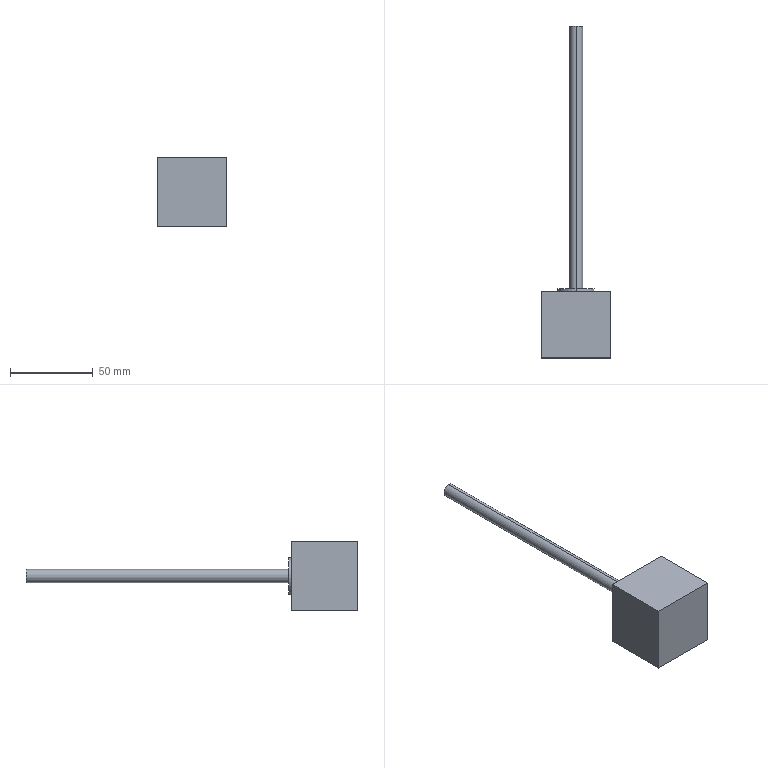Part | SolidWorks | features ICE 3, Extrusion 1, HoleWzd 1 | 1 solid | 28 faces | box 42 x 201 x 42 mm | volume 79160 mm3 | cylinder 12 | cone 8 | plane 8 | commonest cylinder face diameters 2.5 x8 8 x2 22 x2
STEP:
#1=CARTESIAN_POINT('',(-15.5,32.5,-16.75));
#2=VERTEX_POINT('',#1);
#3=CARTESIAN_POINT('',(-15.5,32.5,-14.25));
#4=VERTEX_POINT('',#3);
#5=CARTESIAN_POINT('',(-15.5,32.5,-15.5));
#6=DIRECTION('',(0.,1.,0.));
#7=DIRECTION('',(0.,0.,1.));
#8=AXIS2_PLACEMENT_3D('',#5,#6,#7);
#9=CIRCLE('',#8,1.25);
#10=EDGE_CURVE('',#2,#4,#9,.T.);
#11=ORIENTED_EDGE('',*,*,#10,.F.);
#12=CARTESIAN_POINT('',(-15.5,40.,-16.75));
#13=VERTEX_POINT('',#12);
#14=CARTESIAN_POINT('',(-15.5,40.,-16.75));
#15=DIRECTION('',(0.,1.,0.));
#16=VECTOR('',#15,1000.);
#17=LINE('',#14,#16);
#18=EDGE_CURVE('',#2,#13,#17,.T.);
#19=ORIENTED_EDGE('',*,*,#18,.T.);
#20=CARTESIAN_POINT('',(-15.5,40.,-14.25));
#21=VERTEX_POINT('',#20);
#22=CARTESIAN_POINT('',(-15.5,40.,-15.5));
#23=DIRECTION('',(0.,1.,0.));
#24=DIRECTION('',(0.,0.,1.));
#25=AXIS2_PLACEMENT_3D('',#22,#23,#24);
#26=CIRCLE('',#25,1.25);
#27=EDGE_CURVE('',#13,#21,#26,.T.);
#28=ORIENTED_EDGE('',*,*,#27,.T.);
#29=CARTESIAN_POINT('',(-15.5,40.,-14.25));
#30=DIRECTION('',(0.,1.,0.));
#31=VECTOR('',#30,1000.);
#32=LINE('',#29,#31);
#33=EDGE_CURVE('',#4,#21,#32,.T.);
#34=ORIENTED_EDGE('',*,*,#33,.F.);
#35=EDGE_LOOP('',(#11,#19,#28,#34));
#36=FACE_OUTER_BOUND('',#35,.T.);
#37=CARTESIAN_POINT('',(-15.5,40.,-15.5));
#38=DIRECTION('',(0.,1.,0.));
#39=DIRECTION('',(0.,0.,1.));
#40=AXIS2_PLACEMENT_3D('',#37,#38,#39);
#41=CYLINDRICAL_SURFACE('',#40,1.25);
#42=ADVANCED_FACE('',(#36),#41,.F.);
#43=CARTESIAN_POINT('',(-15.5,31.749,-15.5));
#44=VERTEX_POINT('',#43);
#45=CARTESIAN_POINT('',(-15.5,32.5,-14.25));
#46=DIRECTION('',(0.,0.515,0.8572));
#47=VECTOR('',#46,1000.);
#48=LINE('',#45,#47);
#49=EDGE_CURVE('',#44,#4,#48,.T.);
#50=ORIENTED_EDGE('',*,*,#49,.F.);
#51=CARTESIAN_POINT('',(-15.5,32.5,-16.75));
#52=DIRECTION('',(0.,0.515,-0.8572));
#53=VECTOR('',#52,1000.);
#54=LINE('',#51,#53);
#55=EDGE_CURVE('',#44,#2,#54,.T.);
#56=ORIENTED_EDGE('',*,*,#55,.T.);
#57=ORIENTED_EDGE('',*,*,#10,.T.);
#58=EDGE_LOOP('',(#50,#56,#57));
#59=FACE_OUTER_BOUND('',#58,.T.);
#60=CARTESIAN_POINT('',(-15.5,32.5,-15.5));
#61=DIRECTION('',(0.,1.,0.));
#62=DIRECTION('',(0.,0.,1.));
#63=AXIS2_PLACEMENT_3D('',#60,#61,#62);
#64=CONICAL_SURFACE('',#63,1.25,1.03);
#65=ADVANCED_FACE('',(#59),#64,.F.);
#66=CARTESIAN_POINT('',(15.5,32.5,14.25));
#67=VERTEX_POINT('',#66);
#68=CARTESIAN_POINT('',(15.5,32.5,16.75));
#69=VERTEX_POINT('',#68);
#70=CARTESIAN_POINT('',(15.5,32.5,15.5));
#71=DIRECTION('',(0.,1.,0.));
#72=DIRECTION('',(0.,0.,1.));
#73=AXIS2_PLACEMENT_3D('',#70,#71,#72);
#74=CIRCLE('',#73,1.25);
#75=EDGE_CURVE('',#67,#69,#74,.T.);
#76=ORIENTED_EDGE('',*,*,#75,.F.);
#77=CARTESIAN_POINT('',(15.5,40.,14.25));
#78=VERTEX_POINT('',#77);
#79=CARTESIAN_POINT('',(15.5,40.,14.25));
#80=DIRECTION('',(0.,1.,0.));
#81=VECTOR('',#80,1000.);
#82=LINE('',#79,#81);
#83=EDGE_CURVE('',#67,#78,#82,.T.);
#84=ORIENTED_EDGE('',*,*,#83,.T.);
#85=CARTESIAN_POINT('',(15.5,40.,16.75));
#86=VERTEX_POINT('',#85);
#87=CARTESIAN_POINT('',(15.5,40.,15.5));
#88=DIRECTION('',(0.,1.,0.));
#89=DIRECTION('',(0.,0.,1.));
#90=AXIS2_PLACEMENT_3D('',#87,#88,#89);
#91=CIRCLE('',#90,1.25);
#92=EDGE_CURVE('',#78,#86,#91,.T.);
#93=ORIENTED_EDGE('',*,*,#92,.T.);
#94=CARTESIAN_POINT('',(15.5,40.,16.75));
#95=DIRECTION('',(0.,1.,0.));
#96=VECTOR('',#95,1000.);
#97=LINE('',#94,#96);
#98=EDGE_CURVE('',#69,#86,#97,.T.);
#99=ORIENTED_EDGE('',*,*,#98,.F.);
#100=EDGE_LOOP('',(#76,#84,#93,#99));
#101=FACE_OUTER_BOUND('',#100,.T.);
#102=CARTESIAN_POINT('',(15.5,40.,15.5));
#103=DIRECTION('',(0.,1.,0.));
#104=DIRECTION('',(0.,0.,1.));
#105=AXIS2_PLACEMENT_3D('',#102,#103,#104);
#106=CYLINDRICAL_SURFACE('',#105,1.25);
#107=ADVANCED_FACE('',(#101),#106,.F.);
#108=CARTESIAN_POINT('',(15.5,31.749,15.5));
#109=VERTEX_POINT('',#108);
#110=CARTESIAN_POINT('',(15.5,32.5,16.75));
#111=DIRECTION('',(0.,0.515,0.8572));
#112=VECTOR('',#111,1000.);
#113=LINE('',#110,#112);
#114=EDGE_CURVE('',#109,#69,#113,.T.);
#115=ORIENTED_EDGE('',*,*,#114,.F.);
#116=CARTESIAN_POINT('',(15.5,32.5,14.25));
#117=DIRECTION('',(0.,0.515,-0.8572));
#118=VECTOR('',#117,1000.);
#119=LINE('',#116,#118);
#120=EDGE_CURVE('',#109,#67,#119,.T.);
#121=ORIENTED_EDGE('',*,*,#120,.T.);
#122=ORIENTED_EDGE('',*,*,#75,.T.);
#123=EDGE_LOOP('',(#115,#121,#122));
#124=FACE_OUTER_BOUND('',#123,.T.);
#125=CARTESIAN_POINT('',(15.5,32.5,15.5));
#126=DIRECTION('',(0.,1.,0.));
#127=DIRECTION('',(0.,0.,1.));
#128=AXIS2_PLACEMENT_3D('',#125,#126,#127);
#129=CONICAL_SURFACE('',#128,1.25,1.03);
#130=ADVANCED_FACE('',(#124),#129,.F.);
#131=CARTESIAN_POINT('',(-15.5,32.5,14.25));
#132=VERTEX_POINT('',#131);
#133=CARTESIAN_POINT('',(-15.5,32.5,16.75));
#134=VERTEX_POINT('',#133);
#135=CARTESIAN_POINT('',(-15.5,32.5,15.5));
#136=DIRECTION('',(0.,1.,0.));
#137=DIRECTION('',(0.,0.,1.));
#138=AXIS2_PLACEMENT_3D('',#135,#136,#137);
#139=CIRCLE('',#138,1.25);
#140=EDGE_CURVE('',#132,#134,#139,.T.);
#141=ORIENTED_EDGE('',*,*,#140,.F.);
#142=CARTESIAN_POINT('',(-15.5,40.,14.25));
#143=VERTEX_POINT('',#142);
#144=CARTESIAN_POINT('',(-15.5,40.,14.25));
#145=DIRECTION('',(0.,1.,0.));
#146=VECTOR('',#145,1000.);
#147=LINE('',#144,#146);
#148=EDGE_CURVE('',#132,#143,#147,.T.);
#149=ORIENTED_EDGE('',*,*,#148,.T.);
#150=CARTESIAN_POINT('',(-15.5,40.,16.75));
#151=VERTEX_POINT('',#150);
#152=CARTESIAN_POINT('',(-15.5,40.,15.5));
#153=DIRECTION('',(0.,1.,0.));
#154=DIRECTION('',(0.,0.,1.));
#155=AXIS2_PLACEMENT_3D('',#152,#153,#154);
#156=CIRCLE('',#155,1.25);
#157=EDGE_CURVE('',#143,#151,#156,.T.);
#158=ORIENTED_EDGE('',*,*,#157,.T.);
#159=CARTESIAN_POINT('',(-15.5,40.,16.75));
#160=DIRECTION('',(0.,1.,0.));
#161=VECTOR('',#160,1000.);
#162=LINE('',#159,#161);
#163=EDGE_CURVE('',#134,#151,#162,.T.);
#164=ORIENTED_EDGE('',*,*,#163,.F.);
#165=EDGE_LOOP('',(#141,#149,#158,#164));
#166=FACE_OUTER_BOUND('',#165,.T.);
#167=CARTESIAN_POINT('',(-15.5,40.,15.5));
#168=DIRECTION('',(0.,1.,0.));
#169=DIRECTION('',(0.,0.,1.));
#170=AXIS2_PLACEMENT_3D('',#167,#168,#169);
#171=CYLINDRICAL_SURFACE('',#170,1.25);
#172=ADVANCED_FACE('',(#166),#171,.F.);
#173=CARTESIAN_POINT('',(-15.5,31.749,15.5));
#174=VERTEX_POINT('',#173);
#175=CARTESIAN_POINT('',(-15.5,32.5,16.75));
#176=DIRECTION('',(0.,0.515,0.8572));
#177=VECTOR('',#176,1000.);
#178=LINE('',#175,#177);
#179=EDGE_CURVE('',#174,#134,#178,.T.);
#180=ORIENTED_EDGE('',*,*,#179,.F.);
#181=CARTESIAN_POINT('',(-15.5,32.5,14.25));
#182=DIRECTION('',(0.,0.515,-0.8572));
#183=VECTOR('',#182,1000.);
#184=LINE('',#181,#183);
#185=EDGE_CURVE('',#174,#132,#184,.T.);
#186=ORIENTED_EDGE('',*,*,#185,.T.);
#187=ORIENTED_EDGE('',*,*,#140,.T.);
#188=EDGE_LOOP('',(#180,#186,#187));
#189=FACE_OUTER_BOUND('',#188,.T.);
#190=CARTESIAN_POINT('',(-15.5,32.5,15.5));
#191=DIRECTION('',(0.,1.,0.));
#192=DIRECTION('',(0.,0.,1.));
#193=AXIS2_PLACEMENT_3D('',#190,#191,#192);
#194=CONICAL_SURFACE('',#193,1.25,1.03);
#195=ADVANCED_FACE('',(#189),#194,.F.);
#196=CARTESIAN_POINT('',(15.5,32.5,-16.75));
#197=VERTEX_POINT('',#196);
#198=CARTESIAN_POINT('',(15.5,32.5,-14.25));
#199=VERTEX_POINT('',#198);
#200=CARTESIAN_POINT('',(15.5,32.5,-15.5));
#201=DIRECTION('',(0.,1.,0.));
#202=DIRECTION('',(0.,0.,1.));
#203=AXIS2_PLACEMENT_3D('',#200,#201,#202);
#204=CIRCLE('',#203,1.25);
#205=EDGE_CURVE('',#197,#199,#204,.T.);
#206=ORIENTED_EDGE('',*,*,#205,.F.);
#207=CARTESIAN_POINT('',(15.5,40.,-16.75));
#208=VERTEX_POINT('',#207);
#209=CARTESIAN_POINT('',(15.5,40.,-16.75));
#210=DIRECTION('',(0.,1.,0.));
#211=VECTOR('',#210,1000.);
#212=LINE('',#209,#211);
#213=EDGE_CURVE('',#197,#208,#212,.T.);
#214=ORIENTED_EDGE('',*,*,#213,.T.);
#215=CARTESIAN_POINT('',(15.5,40.,-14.25));
#216=VERTEX_POINT('',#215);
#217=CARTESIAN_POINT('',(15.5,40.,-15.5));
#218=DIRECTION('',(0.,1.,0.));
#219=DIRECTION('',(0.,0.,1.));
#220=AXIS2_PLACEMENT_3D('',#217,#218,#219);
#221=CIRCLE('',#220,1.25);
#222=EDGE_CURVE('',#208,#216,#221,.T.);
#223=ORIENTED_EDGE('',*,*,#222,.T.);
#224=CARTESIAN_POINT('',(15.5,40.,-14.25));
#225=DIRECTION('',(0.,1.,0.));
#226=VECTOR('',#225,1000.);
#227=LINE('',#224,#226);
#228=EDGE_CURVE('',#199,#216,#227,.T.);
#229=ORIENTED_EDGE('',*,*,#228,.F.);
#230=EDGE_LOOP('',(#206,#214,#223,#229));
#231=FACE_OUTER_BOUND('',#230,.T.);
#232=CARTESIAN_POINT('',(15.5,40.,-15.5));
#233=DIRECTION('',(0.,1.,0.));
#234=DIRECTION('',(0.,0.,1.));
#235=AXIS2_PLACEMENT_3D('',#232,#233,#234);
#236=CYLINDRICAL_SURFACE('',#235,1.25);
#237=ADVANCED_FACE('',(#231),#236,.F.);
#238=CARTESIAN_POINT('',(15.5,31.749,-15.5));
#239=VERTEX_POINT('',#238);
#240=CARTESIAN_POINT('',(15.5,32.5,-14.25));
#241=DIRECTION('',(0.,0.515,0.8572));
#242=VECTOR('',#241,1000.);
#243=LINE('',#240,#242);
#244=EDGE_CURVE('',#239,#199,#243,.T.);
#245=ORIENTED_EDGE('',*,*,#244,.F.);
#246=CARTESIAN_POINT('',(15.5,32.5,-16.75));
#247=DIRECTION('',(0.,0.515,-0.8572));
#248=VECTOR('',#247,1000.);
#249=LINE('',#246,#248);
#250=EDGE_CURVE('',#239,#197,#249,.T.);
#251=ORIENTED_EDGE('',*,*,#250,.T.);
#252=ORIENTED_EDGE('',*,*,#205,.T.);
#253=EDGE_LOOP('',(#245,#251,#252));
#254=FACE_OUTER_BOUND('',#253,.T.);
#255=CARTESIAN_POINT('',(15.5,32.5,-15.5));
#256=DIRECTION('',(0.,1.,0.));
#257=DIRECTION('',(0.,0.,1.));
#258=AXIS2_PLACEMENT_3D('',#255,#256,#257);
#259=CONICAL_SURFACE('',#258,1.25,1.03);
#260=ADVANCED_FACE('',(#254),#259,.F.);
#261=CARTESIAN_POINT('',(0.,201.,4.));
#262=VERTEX_POINT('',#261);
#263=CARTESIAN_POINT('',(0.,201.,-4.));
#264=VERTEX_POINT('',#263);
#265=CARTESIAN_POINT('',(0.,201.,0.));
#266=DIRECTION('',(0.,1.,0.));
#267=DIRECTION('',(0.,0.,1.));
#268=AXIS2_PLACEMENT_3D('',#265,#266,#267);
#269=CIRCLE('',#268,4.);
#270=EDGE_CURVE('',#262,#264,#269,.T.);
#271=ORIENTED_EDGE('',*,*,#270,.F.);
#272=CARTESIAN_POINT('',(0.,42.,4.));
#273=VERTEX_POINT('',#272);
#274=CARTESIAN_POINT('',(0.,201.,4.));
#275=DIRECTION('',(0.,-1.,0.));
#276=VECTOR('',#275,1000.);
#277=LINE('',#274,#276);
#278=EDGE_CURVE('',#262,#273,#277,.T.);
#279=ORIENTED_EDGE('',*,*,#278,.T.);
#280=CARTESIAN_POINT('',(0.,42.,-4.));
#281=VERTEX_POINT('',#280);
#282=CARTESIAN_POINT('',(0.,42.,0.));
#283=DIRECTION('',(0.,1.,0.));
#284=DIRECTION('',(0.,0.,1.));
#285=AXIS2_PLACEMENT_3D('',#282,#283,#284);
#286=CIRCLE('',#285,4.);
#287=EDGE_CURVE('',#273,#281,#286,.T.);
#288=ORIENTED_EDGE('',*,*,#287,.T.);
#289=CARTESIAN_POINT('',(0.,201.,-4.));
#290=DIRECTION('',(0.,-1.,0.));
#291=VECTOR('',#290,1000.);
#292=LINE('',#289,#291);
#293=EDGE_CURVE('',#264,#281,#292,.T.);
#294=ORIENTED_EDGE('',*,*,#293,.F.);
#295=EDGE_LOOP('',(#271,#279,#288,#294));
#296=FACE_OUTER_BOUND('',#295,.T.);
#297=CARTESIAN_POINT('',(0.,201.,0.));
#298=DIRECTION('',(0.,-1.,0.));
#299=DIRECTION('',(0.,0.,-1.));
#300=AXIS2_PLACEMENT_3D('',#297,#298,#299);
#301=CYLINDRICAL_SURFACE('',#300,4.);
#302=ADVANCED_FACE('',(#296),#301,.T.);
#303=CARTESIAN_POINT('',(0.,42.,11.));
#304=VERTEX_POINT('',#303);
#305=CARTESIAN_POINT('',(0.,42.,-11.));
#306=VERTEX_POINT('',#305);
#307=CARTESIAN_POINT('',(0.,42.,0.));
#308=DIRECTION('',(0.,1.,0.));
#309=DIRECTION('',(0.,0.,1.));
#310=AXIS2_PLACEMENT_3D('',#307,#308,#309);
#311=CIRCLE('',#310,11.);
#312=EDGE_CURVE('',#304,#306,#311,.T.);
#313=ORIENTED_EDGE('',*,*,#312,.F.);
#314=CARTESIAN_POINT('',(0.,40.,11.));
#315=VERTEX_POINT('',#314);
#316=CARTESIAN_POINT('',(0.,42.,11.));
#317=DIRECTION('',(0.,-1.,0.));
#318=VECTOR('',#317,1000.);
#319=LINE('',#316,#318);
#320=EDGE_CURVE('',#304,#315,#319,.T.);
#321=ORIENTED_EDGE('',*,*,#320,.T.);
#322=CARTESIAN_POINT('',(0.,40.,-11.));
#323=VERTEX_POINT('',#322);
#324=CARTESIAN_POINT('',(0.,40.,0.));
#325=DIRECTION('',(0.,1.,0.));
#326=DIRECTION('',(0.,0.,1.));
#327=AXIS2_PLACEMENT_3D('',#324,#325,#326);
#328=CIRCLE('',#327,11.);
#329=EDGE_CURVE('',#315,#323,#328,.T.);
#330=ORIENTED_EDGE('',*,*,#329,.T.);
#331=CARTESIAN_POINT('',(0.,42.,-11.));
#332=DIRECTION('',(0.,-1.,0.));
#333=VECTOR('',#332,1000.);
#334=LINE('',#331,#333);
#335=EDGE_CURVE('',#306,#323,#334,.T.);
#336=ORIENTED_EDGE('',*,*,#335,.F.);
#337=EDGE_LOOP('',(#313,#321,#330,#336));
#338=FACE_OUTER_BOUND('',#337,.T.);
#339=CARTESIAN_POINT('',(0.,42.,0.));
#340=DIRECTION('',(0.,-1.,0.));
#341=DIRECTION('',(0.,0.,-1.));
#342=AXIS2_PLACEMENT_3D('',#339,#340,#341);
#343=CYLINDRICAL_SURFACE('',#342,11.);
#344=ADVANCED_FACE('',(#338),#343,.T.);
#345=CARTESIAN_POINT('',(21.,0.,21.));
#346=VERTEX_POINT('',#345);
#347=CARTESIAN_POINT('',(21.,0.,-21.));
#348=VERTEX_POINT('',#347);
#349=CARTESIAN_POINT('',(21.,0.,-21.));
#350=DIRECTION('',(0.,0.,-1.));
#351=VECTOR('',#350,1000.);
#352=LINE('',#349,#351);
#353=EDGE_CURVE('',#346,#348,#352,.T.);
#354=ORIENTED_EDGE('',*,*,#353,.T.);
#355=CARTESIAN_POINT('',(21.,40.,-21.));
#356=VERTEX_POINT('',#355);
#357=CARTESIAN_POINT('',(21.,40.,-21.));
#358=DIRECTION('',(0.,-1.,0.));
#359=VECTOR('',#358,1000.);
#360=LINE('',#357,#359);
#361=EDGE_CURVE('',#356,#348,#360,.T.);
#362=ORIENTED_EDGE('',*,*,#361,.F.);
#363=CARTESIAN_POINT('',(21.,40.,21.));
#364=VERTEX_POINT('',#363);
#365=CARTESIAN_POINT('',(21.,40.,-21.));
#366=DIRECTION('',(0.,0.,-1.));
#367=VECTOR('',#366,1000.);
#368=LINE('',#365,#367);
#369=EDGE_CURVE('',#364,#356,#368,.T.);
#370=ORIENTED_EDGE('',*,*,#369,.F.);
#371=CARTESIAN_POINT('',(21.,40.,21.));
#372=DIRECTION('',(0.,-1.,0.));
#373=VECTOR('',#372,1000.);
#374=LINE('',#371,#373);
#375=EDGE_CURVE('',#364,#346,#374,.T.);
#376=ORIENTED_EDGE('',*,*,#375,.T.);
#377=EDGE_LOOP('',(#354,#362,#370,#376));
#378=FACE_OUTER_BOUND('',#377,.T.);
#379=CARTESIAN_POINT('',(21.,40.,-21.));
#380=DIRECTION('',(-1.,0.,0.));
#381=DIRECTION('',(0.,0.,1.));
#382=AXIS2_PLACEMENT_3D('',#379,#380,#381);
#383=PLANE('',#382);
#384=ADVANCED_FACE('',(#378),#383,.F.);
#385=CARTESIAN_POINT('',(-21.,0.,-21.));
#386=VERTEX_POINT('',#385);
#387=CARTESIAN_POINT('',(-21.,0.,-21.));
#388=DIRECTION('',(-1.,0.,0.));
#389=VECTOR('',#388,1000.);
#390=LINE('',#387,#389);
#391=EDGE_CURVE('',#348,#386,#390,.T.);
#392=ORIENTED_EDGE('',*,*,#391,.T.);
#393=CARTESIAN_POINT('',(-21.,40.,-21.));
#394=VERTEX_POINT('',#393);
#395=CARTESIAN_POINT('',(-21.,40.,-21.));
#396=DIRECTION('',(0.,-1.,0.));
#397=VECTOR('',#396,1000.);
#398=LINE('',#395,#397);
#399=EDGE_CURVE('',#394,#386,#398,.T.);
#400=ORIENTED_EDGE('',*,*,#399,.F.);
#401=CARTESIAN_POINT('',(-21.,40.,-21.));
#402=DIRECTION('',(-1.,0.,0.));
#403=VECTOR('',#402,1000.);
#404=LINE('',#401,#403);
#405=EDGE_CURVE('',#356,#394,#404,.T.);
#406=ORIENTED_EDGE('',*,*,#405,.F.);
#407=ORIENTED_EDGE('',*,*,#361,.T.);
#408=EDGE_LOOP('',(#392,#400,#406,#407));
#409=FACE_OUTER_BOUND('',#408,.T.);
#410=CARTESIAN_POINT('',(-21.,40.,-21.));
#411=DIRECTION('',(0.,0.,1.));
#412=DIRECTION('',(1.,0.,0.));
#413=AXIS2_PLACEMENT_3D('',#410,#411,#412);
#414=PLANE('',#413);
#415=ADVANCED_FACE('',(#409),#414,.F.);
#416=CARTESIAN_POINT('',(-21.,0.,21.));
#417=VERTEX_POINT('',#416);
#418=CARTESIAN_POINT('',(-21.,0.,-21.));
#419=DIRECTION('',(0.,0.,1.));
#420=VECTOR('',#419,1000.);
#421=LINE('',#418,#420);
#422=EDGE_CURVE('',#386,#417,#421,.T.);
#423=ORIENTED_EDGE('',*,*,#422,.T.);
#424=CARTESIAN_POINT('',(-21.,40.,21.));
#425=VERTEX_POINT('',#424);
#426=CARTESIAN_POINT('',(-21.,40.,21.));
#427=DIRECTION('',(0.,-1.,0.));
#428=VECTOR('',#427,1000.);
#429=LINE('',#426,#428);
#430=EDGE_CURVE('',#425,#417,#429,.T.);
#431=ORIENTED_EDGE('',*,*,#430,.F.);
#432=CARTESIAN_POINT('',(-21.,40.,-21.));
#433=DIRECTION('',(0.,0.,1.));
#434=VECTOR('',#433,1000.);
#435=LINE('',#432,#434);
#436=EDGE_CURVE('',#394,#425,#435,.T.);
#437=ORIENTED_EDGE('',*,*,#436,.F.);
#438=ORIENTED_EDGE('',*,*,#399,.T.);
#439=EDGE_LOOP('',(#423,#431,#437,#438));
#440=FACE_OUTER_BOUND('',#439,.T.);
#441=CARTESIAN_POINT('',(-21.,40.,-21.));
#442=DIRECTION('',(1.,0.,0.));
#443=DIRECTION('',(0.,0.,-1.));
#444=AXIS2_PLACEMENT_3D('',#441,#442,#443);
#445=PLANE('',#444);
#446=ADVANCED_FACE('',(#440),#445,.F.);
#447=CARTESIAN_POINT('',(-21.,0.,21.));
#448=DIRECTION('',(1.,0.,0.));
#449=VECTOR('',#448,1000.);
#450=LINE('',#447,#449);
#451=EDGE_CURVE('',#417,#346,#450,.T.);
#452=ORIENTED_EDGE('',*,*,#451,.T.);
#453=ORIENTED_EDGE('',*,*,#375,.F.);
#454=CARTESIAN_POINT('',(-21.,40.,21.));
#455=DIRECTION('',(1.,0.,0.));
#456=VECTOR('',#455,1000.);
#457=LINE('',#454,#456);
#458=EDGE_CURVE('',#425,#364,#457,.T.);
#459=ORIENTED_EDGE('',*,*,#458,.F.);
#460=ORIENTED_EDGE('',*,*,#430,.T.);
#461=EDGE_LOOP('',(#452,#453,#459,#460));
#462=FACE_OUTER_BOUND('',#461,.T.);
#463=CARTESIAN_POINT('',(-21.,40.,21.));
#464=DIRECTION('',(0.,0.,-1.));
#465=DIRECTION('',(-1.,0.,0.));
#466=AXIS2_PLACEMENT_3D('',#463,#464,#465);
#467=PLANE('',#466);
#468=ADVANCED_FACE('',(#462),#467,.F.);
#469=CARTESIAN_POINT('',(-15.5,40.,-15.5));
#470=DIRECTION('',(0.,1.,0.));
#471=DIRECTION('',(0.,0.,1.));
#472=AXIS2_PLACEMENT_3D('',#469,#470,#471);
#473=CIRCLE('',#472,1.25);
#474=EDGE_CURVE('',#21,#13,#473,.T.);
#475=ORIENTED_EDGE('',*,*,#474,.F.);
#476=ORIENTED_EDGE('',*,*,#27,.F.);
#477=EDGE_LOOP('',(#475,#476));
#478=FACE_BOUND('',#477,.T.);
#479=CARTESIAN_POINT('',(15.5,40.,15.5));
#480=DIRECTION('',(0.,1.,0.));
#481=DIRECTION('',(0.,0.,1.));
#482=AXIS2_PLACEMENT_3D('',#479,#480,#481);
#483=CIRCLE('',#482,1.25);
#484=EDGE_CURVE('',#86,#78,#483,.T.);
#485=ORIENTED_EDGE('',*,*,#484,.F.);
#486=ORIENTED_EDGE('',*,*,#92,.F.);
#487=EDGE_LOOP('',(#485,#486));
#488=FACE_BOUND('',#487,.T.);
#489=CARTESIAN_POINT('',(-15.5,40.,15.5));
#490=DIRECTION('',(0.,1.,0.));
#491=DIRECTION('',(0.,0.,1.));
#492=AXIS2_PLACEMENT_3D('',#489,#490,#491);
#493=CIRCLE('',#492,1.25);
#494=EDGE_CURVE('',#151,#143,#493,.T.);
#495=ORIENTED_EDGE('',*,*,#494,.F.);
#496=ORIENTED_EDGE('',*,*,#157,.F.);
#497=EDGE_LOOP('',(#495,#496));
#498=FACE_BOUND('',#497,.T.);
#499=CARTESIAN_POINT('',(15.5,40.,-15.5));
#500=DIRECTION('',(0.,1.,0.));
#501=DIRECTION('',(0.,0.,1.));
#502=AXIS2_PLACEMENT_3D('',#499,#500,#501);
#503=CIRCLE('',#502,1.25);
#504=EDGE_CURVE('',#216,#208,#503,.T.);
#505=ORIENTED_EDGE('',*,*,#504,.F.);
#506=ORIENTED_EDGE('',*,*,#222,.F.);
#507=EDGE_LOOP('',(#505,#506));
#508=FACE_BOUND('',#507,.T.);
#509=CARTESIAN_POINT('',(0.,40.,0.));
#510=DIRECTION('',(0.,1.,0.));
#511=DIRECTION('',(0.,0.,1.));
#512=AXIS2_PLACEMENT_3D('',#509,#510,#511);
#513=CIRCLE('',#512,11.);
#514=EDGE_CURVE('',#323,#315,#513,.T.);
#515=ORIENTED_EDGE('',*,*,#514,.F.);
#516=ORIENTED_EDGE('',*,*,#329,.F.);
#517=EDGE_LOOP('',(#515,#516));
#518=FACE_BOUND('',#517,.T.);
#519=ORIENTED_EDGE('',*,*,#369,.T.);
#520=ORIENTED_EDGE('',*,*,#405,.T.);
#521=ORIENTED_EDGE('',*,*,#436,.T.);
#522=ORIENTED_EDGE('',*,*,#458,.T.);
#523=EDGE_LOOP('',(#519,#520,#521,#522));
#524=FACE_OUTER_BOUND('',#523,.T.);
#525=CARTESIAN_POINT('',(0.,40.,0.));
#526=DIRECTION('',(0.,1.,0.));
#527=DIRECTION('',(0.,0.,1.));
#528=AXIS2_PLACEMENT_3D('',#525,#526,#527);
#529=PLANE('',#528);
#530=ADVANCED_FACE('',(#478,#488,#498,#508,#518,#524),#529,.T.);
#531=ORIENTED_EDGE('',*,*,#353,.F.);
#532=ORIENTED_EDGE('',*,*,#451,.F.);
#533=ORIENTED_EDGE('',*,*,#422,.F.);
#534=ORIENTED_EDGE('',*,*,#391,.F.);
#535=EDGE_LOOP('',(#531,#532,#533,#534));
#536=FACE_OUTER_BOUND('',#535,.T.);
#537=CARTESIAN_POINT('',(0.,0.,0.));
#538=DIRECTION('',(0.,1.,0.));
#539=DIRECTION('',(0.,0.,1.));
#540=AXIS2_PLACEMENT_3D('',#537,#538,#539);
#541=PLANE('',#540);
#542=ADVANCED_FACE('',(#536),#541,.F.);
#543=ORIENTED_EDGE('',*,*,#320,.F.);
#544=CARTESIAN_POINT('',(0.,42.,0.));
#545=DIRECTION('',(0.,1.,0.));
#546=DIRECTION('',(0.,0.,1.));
#547=AXIS2_PLACEMENT_3D('',#544,#545,#546);
#548=CIRCLE('',#547,11.);
#549=EDGE_CURVE('',#306,#304,#548,.T.);
#550=ORIENTED_EDGE('',*,*,#549,.F.);
#551=ORIENTED_EDGE('',*,*,#335,.T.);
#552=ORIENTED_EDGE('',*,*,#514,.T.);
#553=EDGE_LOOP('',(#543,#550,#551,#552));
#554=FACE_OUTER_BOUND('',#553,.T.);
#555=CARTESIAN_POINT('',(0.,42.,0.));
#556=DIRECTION('',(0.,-1.,0.));
#557=DIRECTION('',(0.,0.,-1.));
#558=AXIS2_PLACEMENT_3D('',#555,#556,#557);
#559=CYLINDRICAL_SURFACE('',#558,11.);
#560=ADVANCED_FACE('',(#554),#559,.T.);
#561=CARTESIAN_POINT('',(0.,42.,0.));
#562=DIRECTION('',(0.,1.,0.));
#563=DIRECTION('',(0.,0.,1.));
#564=AXIS2_PLACEMENT_3D('',#561,#562,#563);
#565=CIRCLE('',#564,4.);
#566=EDGE_CURVE('',#281,#273,#565,.T.);
#567=ORIENTED_EDGE('',*,*,#566,.F.);
#568=ORIENTED_EDGE('',*,*,#287,.F.);
#569=EDGE_LOOP('',(#567,#568));
#570=FACE_BOUND('',#569,.T.);
#571=ORIENTED_EDGE('',*,*,#549,.T.);
#572=ORIENTED_EDGE('',*,*,#312,.T.);
#573=EDGE_LOOP('',(#571,#572));
#574=FACE_OUTER_BOUND('',#573,.T.);
#575=CARTESIAN_POINT('',(0.,42.,0.));
#576=DIRECTION('',(0.,1.,0.));
#577=DIRECTION('',(0.,0.,1.));
#578=AXIS2_PLACEMENT_3D('',#575,#576,#577);
#579=PLANE('',#578);
#580=ADVANCED_FACE('',(#570,#574),#579,.T.);
#581=ORIENTED_EDGE('',*,*,#278,.F.);
#582=CARTESIAN_POINT('',(0.,201.,0.));
#583=DIRECTION('',(0.,1.,0.));
#584=DIRECTION('',(0.,0.,1.));
#585=AXIS2_PLACEMENT_3D('',#582,#583,#584);
#586=CIRCLE('',#585,4.);
#587=EDGE_CURVE('',#264,#262,#586,.T.);
#588=ORIENTED_EDGE('',*,*,#587,.F.);
#589=ORIENTED_EDGE('',*,*,#293,.T.);
#590=ORIENTED_EDGE('',*,*,#566,.T.);
#591=EDGE_LOOP('',(#581,#588,#589,#590));
#592=FACE_OUTER_BOUND('',#591,.T.);
#593=CARTESIAN_POINT('',(0.,201.,0.));
#594=DIRECTION('',(0.,-1.,0.));
#595=DIRECTION('',(0.,0.,-1.));
#596=AXIS2_PLACEMENT_3D('',#593,#594,#595);
#597=CYLINDRICAL_SURFACE('',#596,4.);
#598=ADVANCED_FACE('',(#592),#597,.T.);
#599=ORIENTED_EDGE('',*,*,#587,.T.);
#600=ORIENTED_EDGE('',*,*,#270,.T.);
#601=EDGE_LOOP('',(#599,#600));
#602=FACE_OUTER_BOUND('',#601,.T.);
#603=CARTESIAN_POINT('',(0.,201.,0.));
#604=DIRECTION('',(0.,1.,0.));
#605=DIRECTION('',(0.,0.,1.));
#606=AXIS2_PLACEMENT_3D('',#603,#604,#605);
#607=PLANE('',#606);
#608=ADVANCED_FACE('',(#602),#607,.T.);
#609=ORIENTED_EDGE('',*,*,#250,.F.);
#610=ORIENTED_EDGE('',*,*,#244,.T.);
#611=CARTESIAN_POINT('',(15.5,32.5,-15.5));
#612=DIRECTION('',(0.,1.,0.));
#613=DIRECTION('',(0.,0.,1.));
#614=AXIS2_PLACEMENT_3D('',#611,#612,#613);
#615=CIRCLE('',#614,1.25);
#616=EDGE_CURVE('',#199,#197,#615,.T.);
#617=ORIENTED_EDGE('',*,*,#616,.T.);
#618=EDGE_LOOP('',(#609,#610,#617));
#619=FACE_OUTER_BOUND('',#618,.T.);
#620=CARTESIAN_POINT('',(15.5,32.5,-15.5));
#621=DIRECTION('',(0.,1.,0.));
#622=DIRECTION('',(0.,0.,1.));
#623=AXIS2_PLACEMENT_3D('',#620,#621,#622);
#624=CONICAL_SURFACE('',#623,1.25,1.03);
#625=ADVANCED_FACE('',(#619),#624,.F.);
#626=ORIENTED_EDGE('',*,*,#213,.F.);
#627=ORIENTED_EDGE('',*,*,#616,.F.);
#628=ORIENTED_EDGE('',*,*,#228,.T.);
#629=ORIENTED_EDGE('',*,*,#504,.T.);
#630=EDGE_LOOP('',(#626,#627,#628,#629));
#631=FACE_OUTER_BOUND('',#630,.T.);
#632=CARTESIAN_POINT('',(15.5,40.,-15.5));
#633=DIRECTION('',(0.,1.,0.));
#634=DIRECTION('',(0.,0.,1.));
#635=AXIS2_PLACEMENT_3D('',#632,#633,#634);
#636=CYLINDRICAL_SURFACE('',#635,1.25);
#637=ADVANCED_FACE('',(#631),#636,.F.);
#638=ORIENTED_EDGE('',*,*,#185,.F.);
#639=ORIENTED_EDGE('',*,*,#179,.T.);
#640=CARTESIAN_POINT('',(-15.5,32.5,15.5));
#641=DIRECTION('',(0.,1.,0.));
#642=DIRECTION('',(0.,0.,1.));
#643=AXIS2_PLACEMENT_3D('',#640,#641,#642);
#644=CIRCLE('',#643,1.25);
#645=EDGE_CURVE('',#134,#132,#644,.T.);
#646=ORIENTED_EDGE('',*,*,#645,.T.);
#647=EDGE_LOOP('',(#638,#639,#646));
#648=FACE_OUTER_BOUND('',#647,.T.);
#649=CARTESIAN_POINT('',(-15.5,32.5,15.5));
#650=DIRECTION('',(0.,1.,0.));
#651=DIRECTION('',(0.,0.,1.));
#652=AXIS2_PLACEMENT_3D('',#649,#650,#651);
#653=CONICAL_SURFACE('',#652,1.25,1.03);
#654=ADVANCED_FACE('',(#648),#653,.F.);
#655=ORIENTED_EDGE('',*,*,#148,.F.);
#656=ORIENTED_EDGE('',*,*,#645,.F.);
#657=ORIENTED_EDGE('',*,*,#163,.T.);
#658=ORIENTED_EDGE('',*,*,#494,.T.);
#659=EDGE_LOOP('',(#655,#656,#657,#658));
#660=FACE_OUTER_BOUND('',#659,.T.);
#661=CARTESIAN_POINT('',(-15.5,40.,15.5));
#662=DIRECTION('',(0.,1.,0.));
#663=DIRECTION('',(0.,0.,1.));
#664=AXIS2_PLACEMENT_3D('',#661,#662,#663);
#665=CYLINDRICAL_SURFACE('',#664,1.25);
#666=ADVANCED_FACE('',(#660),#665,.F.);
#667=ORIENTED_EDGE('',*,*,#120,.F.);
#668=ORIENTED_EDGE('',*,*,#114,.T.);
#669=CARTESIAN_POINT('',(15.5,32.5,15.5));
#670=DIRECTION('',(0.,1.,0.));
#671=DIRECTION('',(0.,0.,1.));
#672=AXIS2_PLACEMENT_3D('',#669,#670,#671);
#673=CIRCLE('',#672,1.25);
#674=EDGE_CURVE('',#69,#67,#673,.T.);
#675=ORIENTED_EDGE('',*,*,#674,.T.);
#676=EDGE_LOOP('',(#667,#668,#675));
#677=FACE_OUTER_BOUND('',#676,.T.);
#678=CARTESIAN_POINT('',(15.5,32.5,15.5));
#679=DIRECTION('',(0.,1.,0.));
#680=DIRECTION('',(0.,0.,1.));
#681=AXIS2_PLACEMENT_3D('',#678,#679,#680);
#682=CONICAL_SURFACE('',#681,1.25,1.03);
#683=ADVANCED_FACE('',(#677),#682,.F.);
#684=ORIENTED_EDGE('',*,*,#83,.F.);
#685=ORIENTED_EDGE('',*,*,#674,.F.);
#686=ORIENTED_EDGE('',*,*,#98,.T.);
#687=ORIENTED_EDGE('',*,*,#484,.T.);
#688=EDGE_LOOP('',(#684,#685,#686,#687));
#689=FACE_OUTER_BOUND('',#688,.T.);
#690=CARTESIAN_POINT('',(15.5,40.,15.5));
#691=DIRECTION('',(0.,1.,0.));
#692=DIRECTION('',(0.,0.,1.));
#693=AXIS2_PLACEMENT_3D('',#690,#691,#692);
#694=CYLINDRICAL_SURFACE('',#693,1.25);
#695=ADVANCED_FACE('',(#689),#694,.F.);
#696=ORIENTED_EDGE('',*,*,#55,.F.);
#697=ORIENTED_EDGE('',*,*,#49,.T.);
#698=CARTESIAN_POINT('',(-15.5,32.5,-15.5));
#699=DIRECTION('',(0.,1.,0.));
#700=DIRECTION('',(0.,0.,1.));
#701=AXIS2_PLACEMENT_3D('',#698,#699,#700);
#702=CIRCLE('',#701,1.25);
#703=EDGE_CURVE('',#4,#2,#702,.T.);
#704=ORIENTED_EDGE('',*,*,#703,.T.);
#705=EDGE_LOOP('',(#696,#697,#704));
#706=FACE_OUTER_BOUND('',#705,.T.);
#707=CARTESIAN_POINT('',(-15.5,32.5,-15.5));
#708=DIRECTION('',(0.,1.,0.));
#709=DIRECTION('',(0.,0.,1.));
#710=AXIS2_PLACEMENT_3D('',#707,#708,#709);
#711=CONICAL_SURFACE('',#710,1.25,1.03);
#712=ADVANCED_FACE('',(#706),#711,.F.);
#713=ORIENTED_EDGE('',*,*,#18,.F.);
#714=ORIENTED_EDGE('',*,*,#703,.F.);
#715=ORIENTED_EDGE('',*,*,#33,.T.);
#716=ORIENTED_EDGE('',*,*,#474,.T.);
#717=EDGE_LOOP('',(#713,#714,#715,#716));
#718=FACE_OUTER_BOUND('',#717,.T.);
#719=CARTESIAN_POINT('',(-15.5,40.,-15.5));
#720=DIRECTION('',(0.,1.,0.));
#721=DIRECTION('',(0.,0.,1.));
#722=AXIS2_PLACEMENT_3D('',#719,#720,#721);
#723=CYLINDRICAL_SURFACE('',#722,1.25);
#724=ADVANCED_FACE('',(#718),#723,.F.);
#725=CLOSED_SHELL('',(#42,#65,#107,#130,#172,#195,#237,#260,#302,#344,#384,#415,#446,#468,#530,#542,#560,#580,#598,#608,#625,#637,#654,#666,#683,#695,#712,#724));
#726=MANIFOLD_SOLID_BREP('',#725);
#727=CARTESIAN_POINT('',(0.,0.,0.));
#728=DIRECTION('',(0.,0.,1.));
#729=DIRECTION('',(1.,0.,0.));
#730=AXIS2_PLACEMENT_3D('',#727,#728,#729);
#731=(LENGTH_UNIT()NAMED_UNIT(*)SI_UNIT(.MILLI.,.METRE.));
#732=UNCERTAINTY_MEASURE_WITH_UNIT(LENGTH_MEASURE(0.00001),#731,'','');
#733=(NAMED_UNIT(*)PLANE_ANGLE_UNIT()SI_UNIT($,.RADIAN.));
#734=(NAMED_UNIT(*)SI_UNIT($,.STERADIAN.)SOLID_ANGLE_UNIT());
#735=(GEOMETRIC_REPRESENTATION_CONTEXT(3)GLOBAL_UNCERTAINTY_ASSIGNED_CONTEXT((#732))GLOBAL_UNIT_ASSIGNED_CONTEXT((#731,#733,#734))REPRESENTATION_CONTEXT('',''));
#736=ADVANCED_BREP_SHAPE_REPRESENTATION('',(#726,#730),#735);